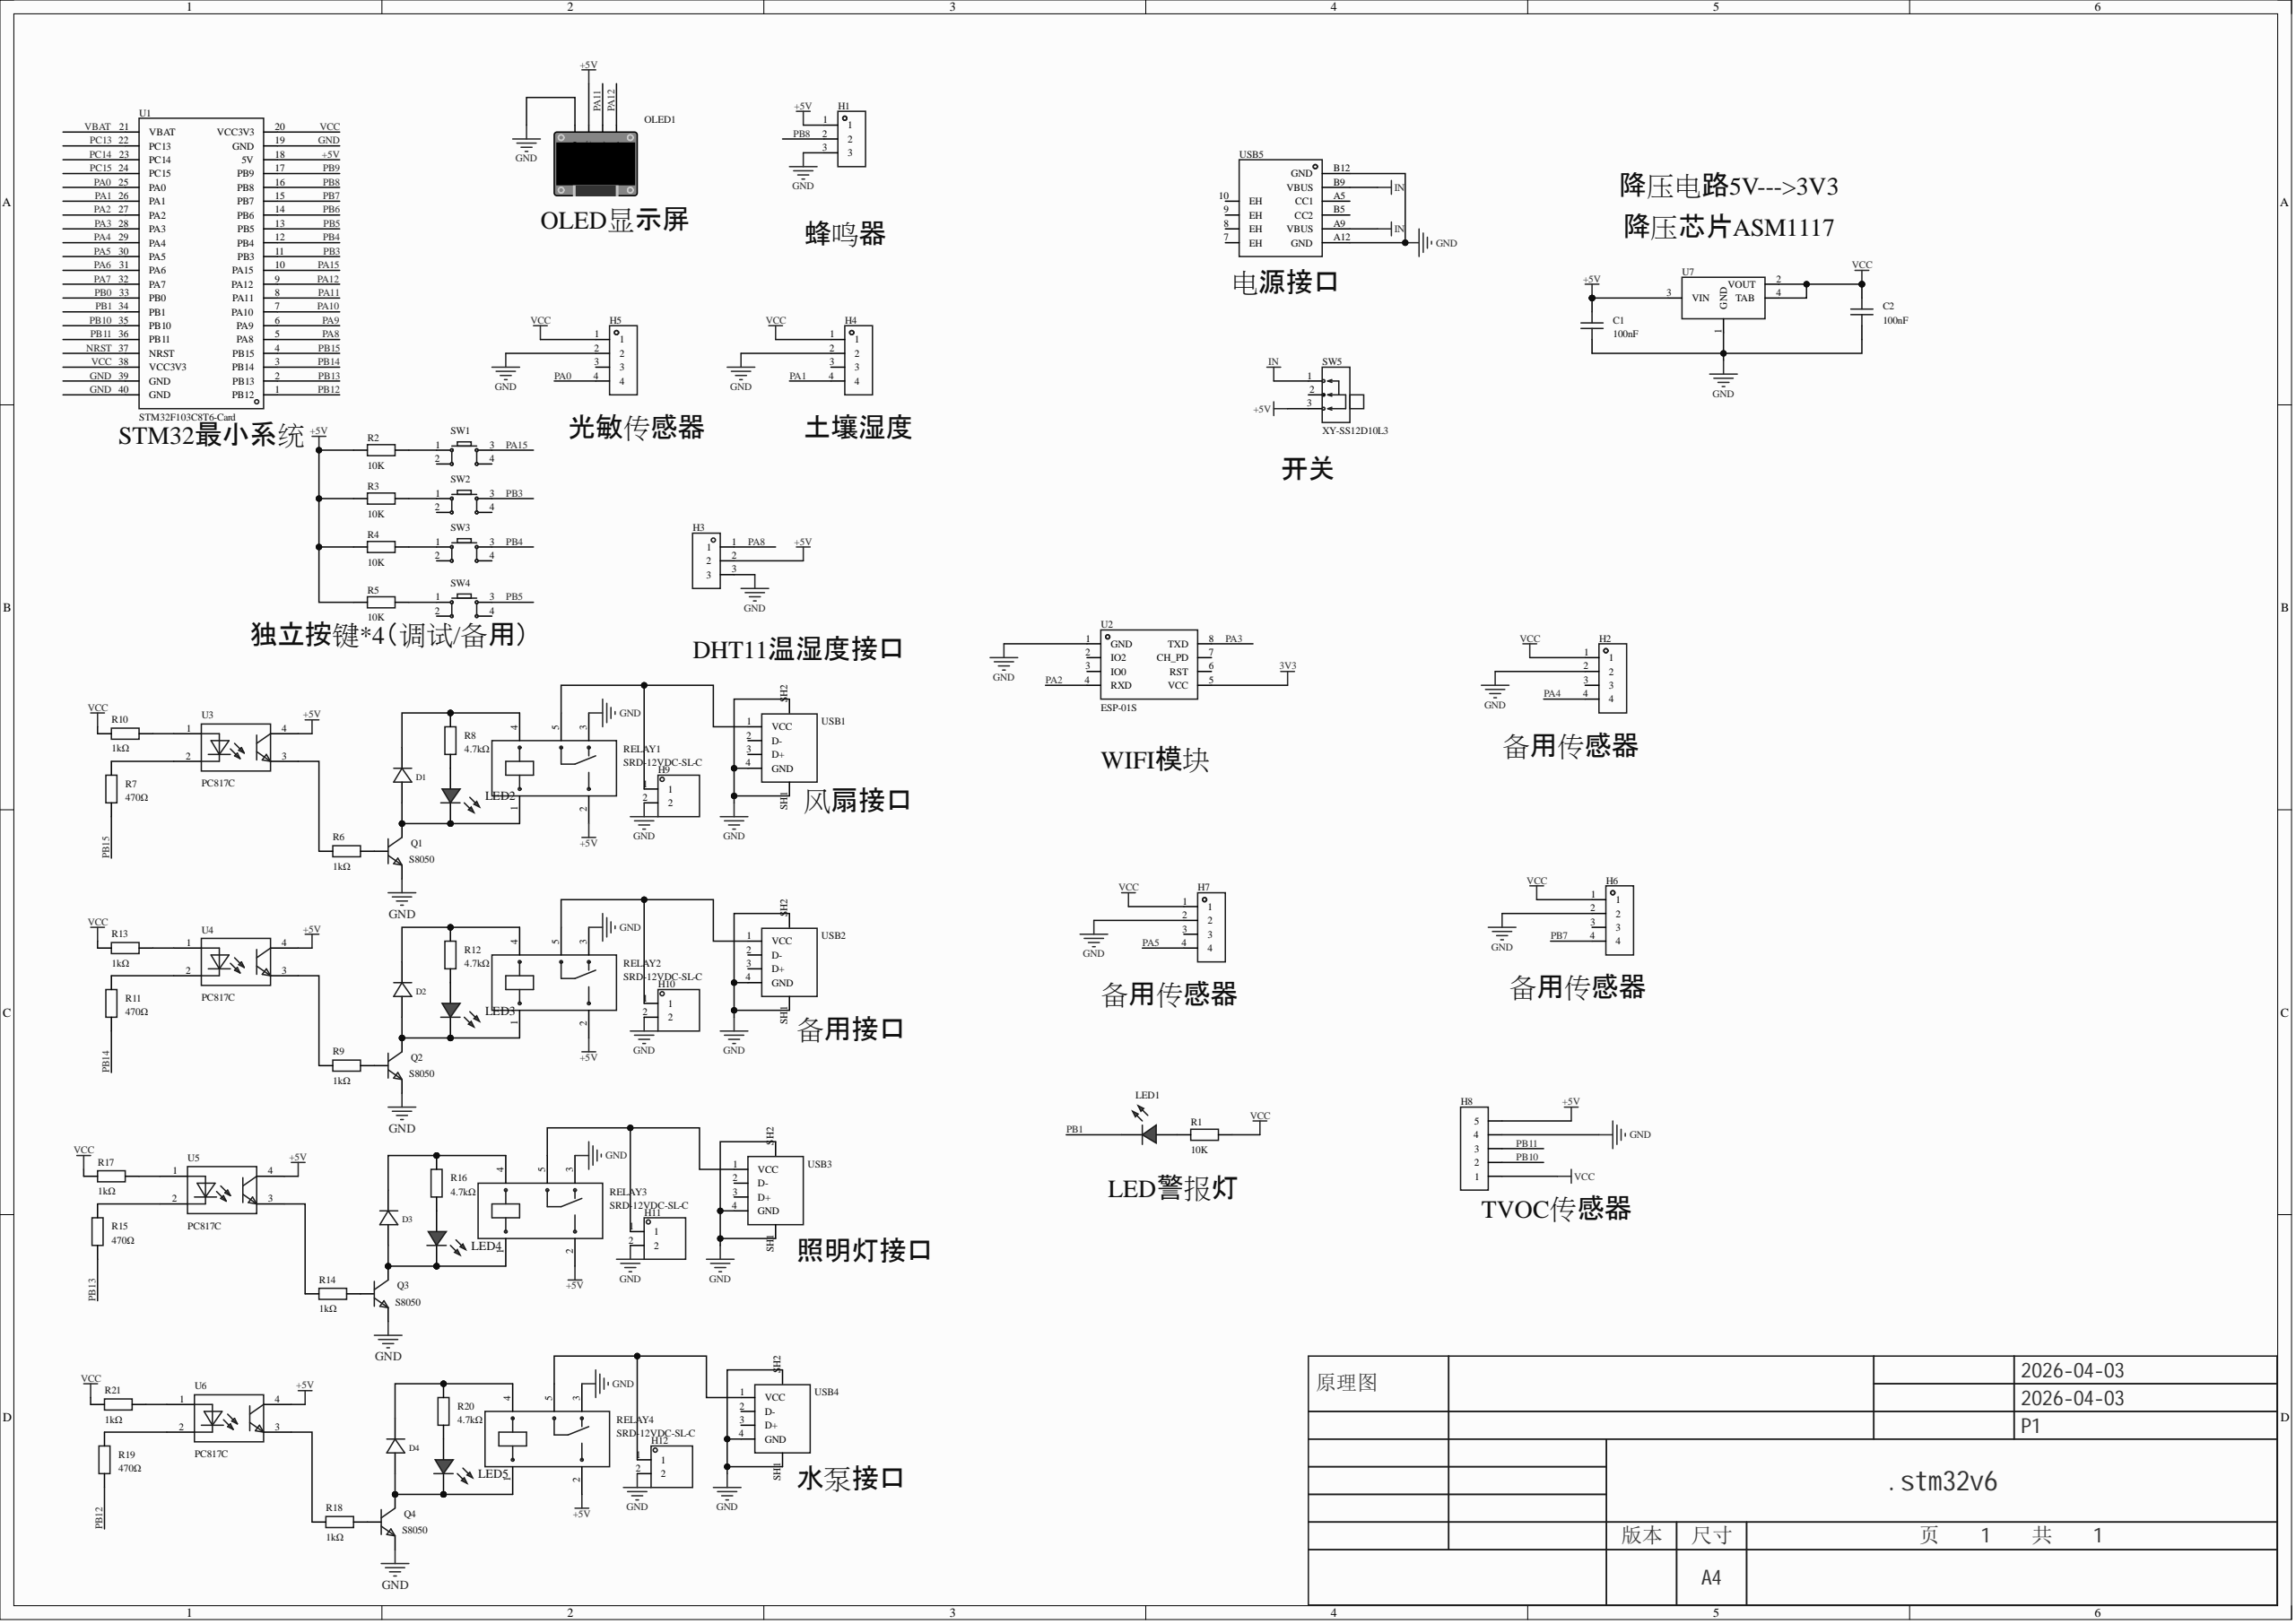Circuit board | Altium Designer | 70 parts | 63 nets
Bill of materials:
Comment,Description,Designator,Footprint,LibRef,Quantity
"100nF","","C1, C2","C0603","CAP_0603","2"
"US1M","二极管配置:独立式;直流反向耐压(Vr):1kV;平均整流电流(Io):1A;正向压降(Vf):1.7V@1A;反向恢复时间(trr):75ns;","D1, D2, D3, D4","SMA_L4.4-W2.8-LS5.4-RD","US1M_C412437","4"
"","","H1, H3","HDR-TH_3P-P2.54-V-F","HDR-F_2.54_1x3P","2"
"","","H2, H4, H5, H6, H7","HDR-TH_4P-P2.54-V-F","HDR-F_2.54_1x4P","5"
"","","H8","HDR-TH_5P-P2.54-V-F","HDR-F_2.54_1x5P","1"
"","","H9, H10, H11, H12","HDR-TH_2P-P2.54-V-M-1","HDR-M_2.54_1x2P","4"
"","","LED1","LED-TH_5mm","LED_TH-R_5mm","1"
"","","LED2, LED3, LED4, LED5","LED_0603","LED_0603-R","4"
"","","OLED1","0.96OLED_4P","0.96OLED模块_4P","1"
"S8050","晶体管类型:NPN;集射极击穿电压(Vceo):25V;集电极电流(Ic):500mA;功率(Pd):300mW;直流电流增益(hFE@Ic,Vce):120@50mA,1V;","Q1, Q2, Q3, Q4","SOT-23-3_L2.9-W1.6-P1.90-LS2.8-BR","S8050_C105433","4"
"10K","","R1, R2, R3, R4, R5","R0603","Res_0603","5"
"1kΩ","","R6, R9, R10, R13, R14, R17, R18, R21","R0603","0603WAF1001T5E","8"
"470Ω","","R7, R11, R15, R19","R0603","0603WAF1001T5E","4"
"4.7kΩ","","R8, R12, R16, R20","R0603","Res_0603","4"
"SRD-12VDC-SL-C","线圈电压:12V;引脚数:5;触点形式:一组转换:1C(单刀双掷-转换);触点容量(电阻负载):-;","RELAY1, RELAY2, RELAY3, RELAY4","RELAY-TH_SRD-XXVDC-XL-C","SRD-12VDC-SL-C","4"
"","","SW1, SW2, SW3, SW4","SW-TH_4P-L6.0-W6.0-P4.50-LS6.5","Key_TH_6x6x6","4"
"XY-SS12D10L3","拨动开关,立式直脚两档,插件,单排正拨,柄长3mm","SW5","SW-TH_3P-L12.7-W6.7_XY-SS12D10LXX","XY-SS12D10L3","1"
"STM32F103C8T6-Card","","U1","CONN-TH_L53.3-W22.9_STM32F103C8T6-CARD","STM32F103C8T6-Card","1"
"ESP-01S","","U2","WIFIM-TH_ESP-01S","ESP-01S_C111009","1"
"PC817C","","U3, U4, U5, U6","OPTO-SMD-4_L4.6-W6.5-P2.54-LS10.3-TL","PC817C_C3025164","4"
"","","U7","SOT_223","AMS1117","1"
"","","USB1, USB2, USB3, USB4","USB_ Type-A","USB_ Type-A","4"
"","","USB5","USB_ TYPE-C-6P","USB_ Type-C-6P","1"
Netlist (Protel format):
[
C1
C0603
100nF



]
[
C2
C0603
100nF



]
[
D1
SMA_L4.4-W2.8-LS5.4-RD
US1M



]
[
D2
SMA_L4.4-W2.8-LS5.4-RD
US1M



]
[
D3
SMA_L4.4-W2.8-LS5.4-RD
US1M



]
[
D4
SMA_L4.4-W2.8-LS5.4-RD
US1M



]
[
H1
HDR-TH_3P-P2.54-V-F




]
[
H2
HDR-TH_4P-P2.54-V-F




]
[
H3
HDR-TH_3P-P2.54-V-F




]
[
H4
HDR-TH_4P-P2.54-V-F




]
[
H5
HDR-TH_4P-P2.54-V-F




]
[
H6
HDR-TH_4P-P2.54-V-F




]
[
H7
HDR-TH_4P-P2.54-V-F




]
[
H8
HDR-TH_5P-P2.54-V-F




]
[
H9
HDR-TH_2P-P2.54-V-M-1




]
[
H10
HDR-TH_2P-P2.54-V-M-1




]
[
H11
HDR-TH_2P-P2.54-V-M-1




]
[
H12
HDR-TH_2P-P2.54-V-M-1




]
[
LED1
LED-TH_5mm




]
[
LED2
LED_0603




]
[
LED3
LED_0603




]
[
LED4
LED_0603




]
[
LED5
LED_0603




]
[
OLED1
0.96OLED_4P




]
[
Q1
SOT-23-3_L2.9-W1.6-P1.90-LS2.8-BR
S8050



]
[
Q2
SOT-23-3_L2.9-W1.6-P1.90-LS2.8-BR
S8050



]
[
Q3
SOT-23-3_L2.9-W1.6-P1.90-LS2.8-BR
S8050



]
[
Q4
SOT-23-3_L2.9-W1.6-P1.90-LS2.8-BR
S8050



]
[
R1
R0603
10K



]
[
R2
R0603
10K



]
[
R3
R0603
10K



]
[
R4
R0603
10K



]
[
R5
R0603
10K



]
[
R6
R0603
1kΩ



]
[
R7
R0603
470Ω



]
[
R8
R0603
4.7kΩ



]
[
R9
R0603
1kΩ



]
[
R10
R0603
1kΩ



]
[
R11
R0603
470Ω



]
[
R12
R0603
4.7kΩ



]
[
R13
R0603
1kΩ



]
[
R14
R0603
1kΩ



]
[
R15
R0603
470Ω



]
[
R16
R0603
4.7kΩ



]
[
R17
R0603
1kΩ



]
[
R18
R0603
1kΩ



]
[
R19
R0603
470Ω



]
[
R20
R0603
4.7kΩ



]
[
R21
R0603
1kΩ



]
[
RELAY1
RELAY-TH_SRD-XXVDC-XL-C
SRD-12VDC-SL-C



]
[
RELAY2
RELAY-TH_SRD-XXVDC-XL-C
SRD-12VDC-SL-C



]
[
RELAY3
RELAY-TH_SRD-XXVDC-XL-C
SRD-12VDC-SL-C



]
[
RELAY4
RELAY-TH_SRD-XXVDC-XL-C
SRD-12VDC-SL-C



]
[
SW1
SW-TH_4P-L6.0-W6.0-P4.50-LS6.5




]
[
SW2
SW-TH_4P-L6.0-W6.0-P4.50-LS6.5




]
[
SW3
SW-TH_4P-L6.0-W6.0-P4.50-LS6.5




]
[
SW4
SW-TH_4P-L6.0-W6.0-P4.50-LS6.5




]
[
SW5
SW-TH_3P-L12.7-W6.7_XY-SS12D10LXX
XY-SS12D10L3



]
[
U1
CONN-TH_L53.3-W22.9_STM32F103C8T6-CARD
STM32F103C8T6-Card



]
[
U2
WIFIM-TH_ESP-01S
ESP-01S



]
[
U3
OPTO-SMD-4_L4.6-W6.5-P2.54-LS10.3-TL
PC817C



]
[
U4
OPTO-SMD-4_L4.6-W6.5-P2.54-LS10.3-TL
PC817C



]
[
U5
OPTO-SMD-4_L4.6-W6.5-P2.54-LS10.3-TL
PC817C



]
[
U6
OPTO-SMD-4_L4.6-W6.5-P2.54-LS10.3-TL
PC817C



]
[
U7
SOT_223




]
[
USB1
USB_ Type-A




]
[
USB2
USB_ Type-A




]
[
USB3
USB_ Type-A




]
[
USB4
USB_ Type-A




]
[
USB5
USB_ TYPE-C-6P




]
(
VCC
C2-2
H2-1
H4-1
H5-1
H6-1
H7-1
H8-1
R1-2
R10-1
R13-1
R17-1
R21-1
U1-20
U1-38
U7-2
U7-4
)
(
PB15
R7-1
U1-4
)
(
PB14
R11-1
U1-3
)
(
PB13
R15-1
U1-2
)
(
PB12
R19-1
U1-1
)
(
PB11
H8-3
U1-36
)
(
PB10
H8-2
U1-35
)
(
PB8
H1-2
U1-16
)
(
PB7
H6-4
U1-15
)
(
PB5
SW4-3
U1-13
)
(
PB4
SW3-3
U1-12
)
(
PB3
SW2-3
U1-11
)
(
PB1
LED1-2
U1-34
)
(
PA15
SW1-3
U1-10
)
(
PA12
OLED1-4
U1-9
)
(
PA11
OLED1-3
U1-8
)
(
PA8
H3-1
U1-5
)
(
PA5
H7-4
U1-30
)
(
PA4
H2-4
U1-29
)
(
PA3
U1-28
U2-8
)
(
PA2
U1-27
U2-4
)
(
PA1
H4-4
U1-26
)
(
PA0
H5-4
U1-25
)
(
NetR21_2
R21-2
U6-1
)
(
NetR19_2
R19-2
U6-2
)
(
NetR18_1
R18-1
U6-3
)
(
NetR17_2
R17-2
U5-1
)
(
NetR15_2
R15-2
U5-2
)
(
NetR14_1
R14-1
U5-3
)
(
NetR13_2
R13-2
U4-1
)
(
NetR11_2
R11-2
U4-2
)
(
NetR10_2
R10-2
U3-1
)
(
NetR9_1
R9-1
U4-3
)
(
NetR7_2
R7-2
U3-2
)
(
NetR6_1
R6-1
U3-3
)
(
NetR5_2
R5-2
SW4-1
)
(
NetR4_2
R4-2
SW3-1
)
(
NetR3_2
R3-2
SW2-1
)
(
NetR2_2
R2-2
SW1-1
)
(
NetQ4_1
Q4-1
R18-2
)
(
NetQ3_1
Q3-1
R14-2
)
(
NetQ2_1
Q2-1
R9-2
)
(
NetQ1_1
Q1-1
R6-2
)
(
NetLED5_2
LED5-2
R20-1
)
(
NetLED4_2
LED4-2
R16-1
)
(
NetLED3_2
LED3-2
R12-1
)
(
NetLED2_2
LED2-2
R8-1
)
(
NetLED1_1
LED1-1
R1-1
)
(
NetH12_1
H12-1
RELAY4-5
USB4-1
)
(
NetH11_1
H11-1
RELAY3-5
USB3-1
)
(
NetH10_1
H10-1
RELAY2-5
USB2-1
)
(
NetH9_1
H9-1
RELAY1-5
USB1-1
)
(
NetD4_2
D4-2
LED5-1
Q4-3
RELAY4-1
)
(
NetD4_1
D4-1
R20-2
RELAY4-4
)
(
NetD3_2
D3-2
LED4-1
Q3-3
RELAY3-1
)
(
NetD3_1
D3-1
R16-2
RELAY3-4
)
(
NetD2_2
D2-2
LED3-1
Q2-3
RELAY2-1
)
(
NetD2_1
D2-1
R12-2
RELAY2-4
)
(
NetD1_2
D1-2
LED2-1
Q1-3
RELAY1-1
)
(
NetD1_1
D1-1
R8-2
RELAY1-4
)
(
IN
SW5-1
USB5-A9
USB5-B9
)
(
GND
C1-1
C2-1
H1-3
H2-2
H3-3
H4-2
H5-2
H6-2
H7-2
H8-4
H9-2
H10-2
H11-2
H12-2
OLED1-1
Q1-2
Q2-2
Q3-2
Q4-2
RELAY1-3
RELAY2-3
RELAY3-3
RELAY4-3
U1-19
U1-39
U1-40
U2-1
U7-1
USB1-4
USB1-SH1
USB1-SH2
USB2-4
USB2-SH1
USB2-SH2
USB3-4
USB3-SH1
USB3-SH2
USB4-4
USB4-SH1
USB4-SH2
USB5-A12
USB5-B12
)
(
+5V
C1-2
H1-1
H3-2
H8-5
OLED1-2
R2-1
R3-1
R4-1
R5-1
RELAY1-2
RELAY2-2
RELAY3-2
RELAY4-2
SW5-3
U1-18
U3-4
U4-4
U5-4
U6-4
U7-3
)